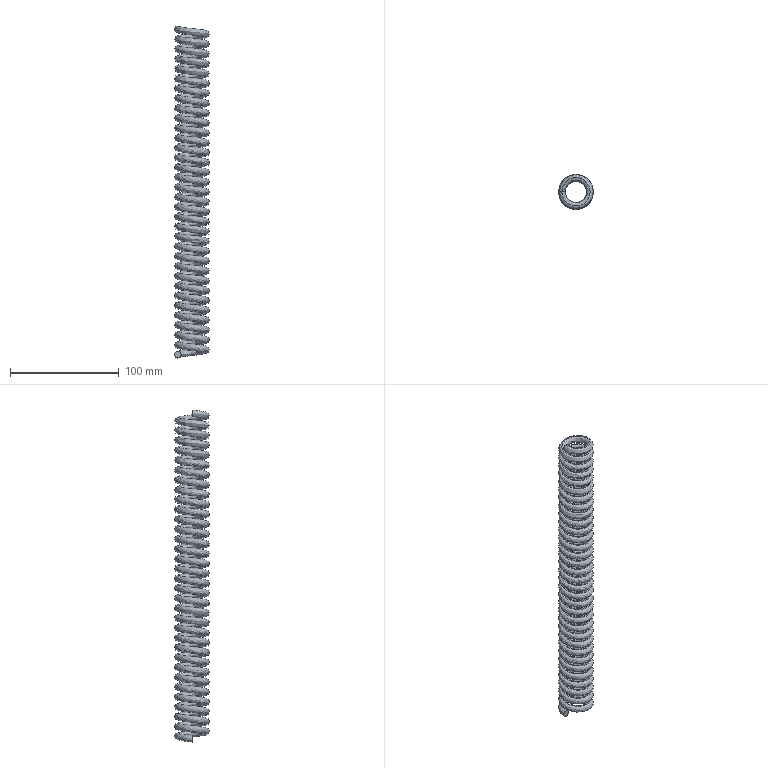Part | SolidWorks | features Helix 1, RefAxis 1, Sweep 1 | 1 solid | 4 faces | box 32 x 32 x 306 mm | volume 76200 mm3 | spline 2 | plane 2